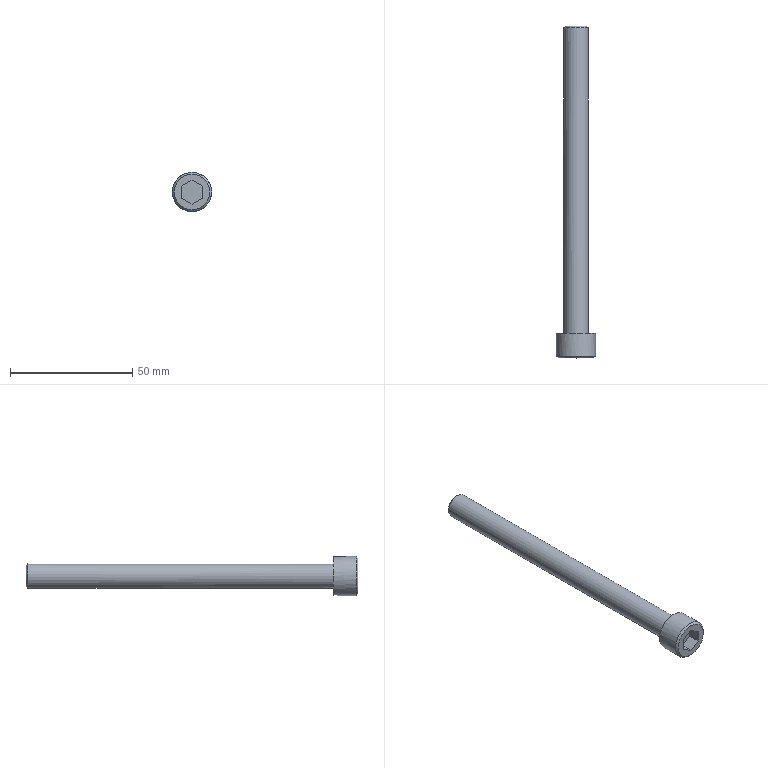Part | NX | features M10.00-135.00 2 | 1 solid | 14 faces | box 16 x 135.5 x 16 mm | volume 11532 mm3 | plane 10 | cylinder 2 | cone 2 | commonest cylinder face diameters 10 x1 16 x1
STEP:
#1=CARTESIAN_POINT('',(60.,-290.5,-15.25));
#2=VERTEX_POINT('',#1);
#3=CARTESIAN_POINT('',(60.,-290.5,-22.5));
#4=DIRECTION('',(0.,1.,0.));
#5=DIRECTION('',(0.,0.,1.));
#6=AXIS2_PLACEMENT_3D('',#3,#4,#5);
#7=CIRCLE('',#6,7.25);
#8=EDGE_CURVE('',#2,#2,#7,.T.);
#9=ORIENTED_EDGE('',*,*,#8,.F.);
#10=EDGE_LOOP('',(#9));
#11=FACE_BOUND('',#10,.T.);
#12=CARTESIAN_POINT('',(55.75,-290.5,-24.954));
#13=VERTEX_POINT('',#12);
#14=CARTESIAN_POINT('',(55.75,-290.5,-20.046));
#15=VERTEX_POINT('',#14);
#16=CARTESIAN_POINT('',(55.75,-290.5,-24.954));
#17=DIRECTION('',(0.,0.,1.));
#18=VECTOR('',#17,1000.);
#19=LINE('',#16,#18);
#20=EDGE_CURVE('',#13,#15,#19,.T.);
#21=ORIENTED_EDGE('',*,*,#20,.T.);
#22=CARTESIAN_POINT('',(60.,-290.5,-17.593));
#23=VERTEX_POINT('',#22);
#24=CARTESIAN_POINT('',(55.75,-290.5,-20.046));
#25=DIRECTION('',(0.866,0.,0.5));
#26=VECTOR('',#25,1000.);
#27=LINE('',#24,#26);
#28=EDGE_CURVE('',#15,#23,#27,.T.);
#29=ORIENTED_EDGE('',*,*,#28,.T.);
#30=CARTESIAN_POINT('',(64.25,-290.5,-20.046));
#31=VERTEX_POINT('',#30);
#32=CARTESIAN_POINT('',(60.,-290.5,-17.593));
#33=DIRECTION('',(0.866,0.,-0.5));
#34=VECTOR('',#33,1000.);
#35=LINE('',#32,#34);
#36=EDGE_CURVE('',#23,#31,#35,.T.);
#37=ORIENTED_EDGE('',*,*,#36,.T.);
#38=CARTESIAN_POINT('',(64.25,-290.5,-24.954));
#39=VERTEX_POINT('',#38);
#40=CARTESIAN_POINT('',(64.25,-290.5,-20.046));
#41=DIRECTION('',(0.,0.,-1.));
#42=VECTOR('',#41,1000.);
#43=LINE('',#40,#42);
#44=EDGE_CURVE('',#31,#39,#43,.T.);
#45=ORIENTED_EDGE('',*,*,#44,.T.);
#46=CARTESIAN_POINT('',(60.,-290.5,-27.407));
#47=VERTEX_POINT('',#46);
#48=CARTESIAN_POINT('',(64.25,-290.5,-24.954));
#49=DIRECTION('',(-0.866,0.,-0.5));
#50=VECTOR('',#49,1000.);
#51=LINE('',#48,#50);
#52=EDGE_CURVE('',#39,#47,#51,.T.);
#53=ORIENTED_EDGE('',*,*,#52,.T.);
#54=CARTESIAN_POINT('',(60.,-290.5,-27.407));
#55=DIRECTION('',(-0.866,0.,0.5));
#56=VECTOR('',#55,1000.);
#57=LINE('',#54,#56);
#58=EDGE_CURVE('',#47,#13,#57,.T.);
#59=ORIENTED_EDGE('',*,*,#58,.T.);
#60=EDGE_LOOP('',(#21,#29,#37,#45,#53,#59));
#61=FACE_BOUND('',#60,.T.);
#62=CARTESIAN_POINT('',(60.,-290.5,-22.5));
#63=DIRECTION('',(0.,-1.,0.));
#64=DIRECTION('',(0.,0.,1.));
#65=AXIS2_PLACEMENT_3D('',#62,#63,#64);
#66=PLANE('',#65);
#67=ADVANCED_FACE('',(#11,#61),#66,.T.);
#68=CARTESIAN_POINT('',(65.,-280.5,-22.5));
#69=VERTEX_POINT('',#68);
#70=CARTESIAN_POINT('',(60.,-280.5,-22.5));
#71=DIRECTION('',(0.,-1.,0.));
#72=DIRECTION('',(1.,0.,0.));
#73=AXIS2_PLACEMENT_3D('',#70,#71,#72);
#74=CIRCLE('',#73,5.);
#75=EDGE_CURVE('',#69,#69,#74,.T.);
#76=ORIENTED_EDGE('',*,*,#75,.T.);
#77=EDGE_LOOP('',(#76));
#78=FACE_BOUND('',#77,.T.);
#79=CARTESIAN_POINT('',(68.,-280.5,-22.5));
#80=VERTEX_POINT('',#79);
#81=CARTESIAN_POINT('',(60.,-280.5,-22.5));
#82=DIRECTION('',(0.,1.,0.));
#83=DIRECTION('',(1.,0.,0.));
#84=AXIS2_PLACEMENT_3D('',#81,#82,#83);
#85=CIRCLE('',#84,8.);
#86=EDGE_CURVE('',#80,#80,#85,.T.);
#87=ORIENTED_EDGE('',*,*,#86,.T.);
#88=EDGE_LOOP('',(#87));
#89=FACE_BOUND('',#88,.T.);
#90=CARTESIAN_POINT('',(60.,-280.5,-22.5));
#91=DIRECTION('',(0.,1.,0.));
#92=DIRECTION('',(0.,0.,-1.));
#93=AXIS2_PLACEMENT_3D('',#90,#91,#92);
#94=PLANE('',#93);
#95=ADVANCED_FACE('',(#78,#89),#94,.T.);
#96=CARTESIAN_POINT('',(60.,-289.75,-14.5));
#97=VERTEX_POINT('',#96);
#98=CARTESIAN_POINT('',(60.,-289.75,-22.5));
#99=DIRECTION('',(0.,1.,0.));
#100=DIRECTION('',(0.,0.,1.));
#101=AXIS2_PLACEMENT_3D('',#98,#99,#100);
#102=CIRCLE('',#101,8.);
#103=EDGE_CURVE('',#97,#97,#102,.F.);
#104=ORIENTED_EDGE('',*,*,#103,.F.);
#105=EDGE_LOOP('',(#104));
#106=FACE_BOUND('',#105,.T.);
#107=ORIENTED_EDGE('',*,*,#86,.F.);
#108=EDGE_LOOP('',(#107));
#109=FACE_BOUND('',#108,.T.);
#110=CARTESIAN_POINT('',(60.,-280.5,-22.5));
#111=DIRECTION('',(0.,-1.,0.));
#112=DIRECTION('',(1.,0.,0.));
#113=AXIS2_PLACEMENT_3D('',#110,#111,#112);
#114=CYLINDRICAL_SURFACE('',#113,8.);
#115=ADVANCED_FACE('',(#106,#109),#114,.T.);
#116=CARTESIAN_POINT('',(60.,-155.,-26.75));
#117=VERTEX_POINT('',#116);
#118=CARTESIAN_POINT('',(60.,-155.,-22.5));
#119=DIRECTION('',(0.,-1.,0.));
#120=DIRECTION('',(0.,0.,-1.));
#121=AXIS2_PLACEMENT_3D('',#118,#119,#120);
#122=CIRCLE('',#121,4.25);
#123=EDGE_CURVE('',#117,#117,#122,.T.);
#124=ORIENTED_EDGE('',*,*,#123,.F.);
#125=EDGE_LOOP('',(#124));
#126=FACE_BOUND('',#125,.T.);
#127=CARTESIAN_POINT('',(60.,-155.,-22.5));
#128=DIRECTION('',(0.,1.,0.));
#129=DIRECTION('',(0.,0.,-1.));
#130=AXIS2_PLACEMENT_3D('',#127,#128,#129);
#131=PLANE('',#130);
#132=ADVANCED_FACE('',(#126),#131,.T.);
#133=CARTESIAN_POINT('',(60.,-155.75,-27.5));
#134=VERTEX_POINT('',#133);
#135=CARTESIAN_POINT('',(60.,-155.75,-22.5));
#136=DIRECTION('',(0.,-1.,0.));
#137=DIRECTION('',(0.,0.,-1.));
#138=AXIS2_PLACEMENT_3D('',#135,#136,#137);
#139=CIRCLE('',#138,5.);
#140=EDGE_CURVE('',#134,#134,#139,.F.);
#141=ORIENTED_EDGE('',*,*,#140,.F.);
#142=EDGE_LOOP('',(#141));
#143=FACE_BOUND('',#142,.T.);
#144=ORIENTED_EDGE('',*,*,#75,.F.);
#145=EDGE_LOOP('',(#144));
#146=FACE_BOUND('',#145,.T.);
#147=CARTESIAN_POINT('',(60.,-280.5,-22.5));
#148=DIRECTION('',(0.,1.,0.));
#149=DIRECTION('',(1.,0.,0.));
#150=AXIS2_PLACEMENT_3D('',#147,#148,#149);
#151=CYLINDRICAL_SURFACE('',#150,5.);
#152=ADVANCED_FACE('',(#143,#146),#151,.T.);
#153=ORIENTED_EDGE('',*,*,#28,.F.);
#154=CARTESIAN_POINT('',(55.75,-285.5,-20.046));
#155=VERTEX_POINT('',#154);
#156=CARTESIAN_POINT('',(55.75,-285.5,-20.046));
#157=DIRECTION('',(0.,-1.,0.));
#158=VECTOR('',#157,1000.);
#159=LINE('',#156,#158);
#160=EDGE_CURVE('',#15,#155,#159,.F.);
#161=ORIENTED_EDGE('',*,*,#160,.T.);
#162=CARTESIAN_POINT('',(60.,-285.5,-17.593));
#163=VERTEX_POINT('',#162);
#164=CARTESIAN_POINT('',(55.75,-285.5,-20.046));
#165=DIRECTION('',(0.866,0.,0.5));
#166=VECTOR('',#165,1000.);
#167=LINE('',#164,#166);
#168=EDGE_CURVE('',#163,#155,#167,.F.);
#169=ORIENTED_EDGE('',*,*,#168,.F.);
#170=CARTESIAN_POINT('',(60.,-285.5,-17.593));
#171=DIRECTION('',(0.,-1.,0.));
#172=VECTOR('',#171,1000.);
#173=LINE('',#170,#172);
#174=EDGE_CURVE('',#23,#163,#173,.F.);
#175=ORIENTED_EDGE('',*,*,#174,.F.);
#176=EDGE_LOOP('',(#153,#161,#169,#175));
#177=FACE_BOUND('',#176,.T.);
#178=CARTESIAN_POINT('',(57.875,-288.,-18.819));
#179=DIRECTION('',(-0.5,0.,0.866));
#180=DIRECTION('',(0.866,0.,0.5));
#181=AXIS2_PLACEMENT_3D('',#178,#179,#180);
#182=PLANE('',#181);
#183=ADVANCED_FACE('',(#177),#182,.F.);
#184=ORIENTED_EDGE('',*,*,#20,.F.);
#185=CARTESIAN_POINT('',(55.75,-285.5,-24.954));
#186=VERTEX_POINT('',#185);
#187=CARTESIAN_POINT('',(55.75,-285.5,-24.954));
#188=DIRECTION('',(0.,-1.,0.));
#189=VECTOR('',#188,1000.);
#190=LINE('',#187,#189);
#191=EDGE_CURVE('',#13,#186,#190,.F.);
#192=ORIENTED_EDGE('',*,*,#191,.T.);
#193=CARTESIAN_POINT('',(55.75,-285.5,-24.954));
#194=DIRECTION('',(0.,0.,1.));
#195=VECTOR('',#194,1000.);
#196=LINE('',#193,#195);
#197=EDGE_CURVE('',#155,#186,#196,.F.);
#198=ORIENTED_EDGE('',*,*,#197,.F.);
#199=ORIENTED_EDGE('',*,*,#160,.F.);
#200=EDGE_LOOP('',(#184,#192,#198,#199));
#201=FACE_BOUND('',#200,.T.);
#202=CARTESIAN_POINT('',(55.75,-288.,-22.5));
#203=DIRECTION('',(-1.,0.,0.));
#204=DIRECTION('',(0.,1.,0.));
#205=AXIS2_PLACEMENT_3D('',#202,#203,#204);
#206=PLANE('',#205);
#207=ADVANCED_FACE('',(#201),#206,.F.);
#208=ORIENTED_EDGE('',*,*,#58,.F.);
#209=CARTESIAN_POINT('',(60.,-285.5,-27.407));
#210=VERTEX_POINT('',#209);
#211=CARTESIAN_POINT('',(60.,-285.5,-27.407));
#212=DIRECTION('',(0.,-1.,0.));
#213=VECTOR('',#212,1000.);
#214=LINE('',#211,#213);
#215=EDGE_CURVE('',#47,#210,#214,.F.);
#216=ORIENTED_EDGE('',*,*,#215,.T.);
#217=CARTESIAN_POINT('',(60.,-285.5,-27.407));
#218=DIRECTION('',(-0.866,0.,0.5));
#219=VECTOR('',#218,1000.);
#220=LINE('',#217,#219);
#221=EDGE_CURVE('',#186,#210,#220,.F.);
#222=ORIENTED_EDGE('',*,*,#221,.F.);
#223=ORIENTED_EDGE('',*,*,#191,.F.);
#224=EDGE_LOOP('',(#208,#216,#222,#223));
#225=FACE_BOUND('',#224,.T.);
#226=CARTESIAN_POINT('',(57.875,-288.,-26.181));
#227=DIRECTION('',(-0.5,0.,-0.866));
#228=DIRECTION('',(-0.866,0.,0.5));
#229=AXIS2_PLACEMENT_3D('',#226,#227,#228);
#230=PLANE('',#229);
#231=ADVANCED_FACE('',(#225),#230,.F.);
#232=ORIENTED_EDGE('',*,*,#52,.F.);
#233=CARTESIAN_POINT('',(64.25,-285.5,-24.954));
#234=VERTEX_POINT('',#233);
#235=CARTESIAN_POINT('',(64.25,-285.5,-24.954));
#236=DIRECTION('',(0.,-1.,0.));
#237=VECTOR('',#236,1000.);
#238=LINE('',#235,#237);
#239=EDGE_CURVE('',#39,#234,#238,.F.);
#240=ORIENTED_EDGE('',*,*,#239,.T.);
#241=CARTESIAN_POINT('',(64.25,-285.5,-24.954));
#242=DIRECTION('',(-0.866,0.,-0.5));
#243=VECTOR('',#242,1000.);
#244=LINE('',#241,#243);
#245=EDGE_CURVE('',#210,#234,#244,.F.);
#246=ORIENTED_EDGE('',*,*,#245,.F.);
#247=ORIENTED_EDGE('',*,*,#215,.F.);
#248=EDGE_LOOP('',(#232,#240,#246,#247));
#249=FACE_BOUND('',#248,.T.);
#250=CARTESIAN_POINT('',(62.125,-288.,-26.181));
#251=DIRECTION('',(0.5,0.,-0.866));
#252=DIRECTION('',(-0.866,0.,-0.5));
#253=AXIS2_PLACEMENT_3D('',#250,#251,#252);
#254=PLANE('',#253);
#255=ADVANCED_FACE('',(#249),#254,.F.);
#256=ORIENTED_EDGE('',*,*,#44,.F.);
#257=CARTESIAN_POINT('',(64.25,-285.5,-20.046));
#258=VERTEX_POINT('',#257);
#259=CARTESIAN_POINT('',(64.25,-285.5,-20.046));
#260=DIRECTION('',(0.,-1.,0.));
#261=VECTOR('',#260,1000.);
#262=LINE('',#259,#261);
#263=EDGE_CURVE('',#31,#258,#262,.F.);
#264=ORIENTED_EDGE('',*,*,#263,.T.);
#265=CARTESIAN_POINT('',(64.25,-285.5,-20.046));
#266=DIRECTION('',(0.,0.,-1.));
#267=VECTOR('',#266,1000.);
#268=LINE('',#265,#267);
#269=EDGE_CURVE('',#234,#258,#268,.F.);
#270=ORIENTED_EDGE('',*,*,#269,.F.);
#271=ORIENTED_EDGE('',*,*,#239,.F.);
#272=EDGE_LOOP('',(#256,#264,#270,#271));
#273=FACE_BOUND('',#272,.T.);
#274=CARTESIAN_POINT('',(64.25,-288.,-22.5));
#275=DIRECTION('',(1.,0.,0.));
#276=DIRECTION('',(0.,-1.,0.));
#277=AXIS2_PLACEMENT_3D('',#274,#275,#276);
#278=PLANE('',#277);
#279=ADVANCED_FACE('',(#273),#278,.F.);
#280=ORIENTED_EDGE('',*,*,#36,.F.);
#281=ORIENTED_EDGE('',*,*,#174,.T.);
#282=CARTESIAN_POINT('',(60.,-285.5,-17.593));
#283=DIRECTION('',(0.866,0.,-0.5));
#284=VECTOR('',#283,1000.);
#285=LINE('',#282,#284);
#286=EDGE_CURVE('',#258,#163,#285,.F.);
#287=ORIENTED_EDGE('',*,*,#286,.F.);
#288=ORIENTED_EDGE('',*,*,#263,.F.);
#289=EDGE_LOOP('',(#280,#281,#287,#288));
#290=FACE_BOUND('',#289,.T.);
#291=CARTESIAN_POINT('',(62.125,-288.,-18.819));
#292=DIRECTION('',(0.5,0.,0.866));
#293=DIRECTION('',(0.866,0.,-0.5));
#294=AXIS2_PLACEMENT_3D('',#291,#292,#293);
#295=PLANE('',#294);
#296=ADVANCED_FACE('',(#290),#295,.F.);
#297=ORIENTED_EDGE('',*,*,#286,.T.);
#298=ORIENTED_EDGE('',*,*,#168,.T.);
#299=ORIENTED_EDGE('',*,*,#197,.T.);
#300=ORIENTED_EDGE('',*,*,#221,.T.);
#301=ORIENTED_EDGE('',*,*,#245,.T.);
#302=ORIENTED_EDGE('',*,*,#269,.T.);
#303=EDGE_LOOP('',(#297,#298,#299,#300,#301,#302));
#304=FACE_BOUND('',#303,.T.);
#305=CARTESIAN_POINT('',(60.,-285.5,-22.5));
#306=DIRECTION('',(0.,1.,0.));
#307=DIRECTION('',(0.,0.,-1.));
#308=AXIS2_PLACEMENT_3D('',#305,#306,#307);
#309=PLANE('',#308);
#310=ADVANCED_FACE('',(#304),#309,.F.);
#311=ORIENTED_EDGE('',*,*,#123,.T.);
#312=EDGE_LOOP('',(#311));
#313=FACE_BOUND('',#312,.T.);
#314=ORIENTED_EDGE('',*,*,#140,.T.);
#315=EDGE_LOOP('',(#314));
#316=FACE_BOUND('',#315,.T.);
#317=CARTESIAN_POINT('',(60.,-155.75,-22.5));
#318=DIRECTION('',(0.,-1.,0.));
#319=DIRECTION('',(0.,0.,1.));
#320=AXIS2_PLACEMENT_3D('',#317,#318,#319);
#321=CONICAL_SURFACE('',#320,5.,0.7854);
#322=ADVANCED_FACE('',(#313,#316),#321,.T.);
#323=ORIENTED_EDGE('',*,*,#8,.T.);
#324=EDGE_LOOP('',(#323));
#325=FACE_BOUND('',#324,.T.);
#326=ORIENTED_EDGE('',*,*,#103,.T.);
#327=EDGE_LOOP('',(#326));
#328=FACE_BOUND('',#327,.T.);
#329=CARTESIAN_POINT('',(60.,-289.75,-22.5));
#330=DIRECTION('',(0.,1.,0.));
#331=DIRECTION('',(0.,0.,-1.));
#332=AXIS2_PLACEMENT_3D('',#329,#330,#331);
#333=CONICAL_SURFACE('',#332,8.,0.7854);
#334=ADVANCED_FACE('',(#325,#328),#333,.T.);
#335=CLOSED_SHELL('',(#67,#95,#115,#132,#152,#183,#207,#231,#255,#279,#296,#310,#322,#334));
#336=MANIFOLD_SOLID_BREP('',#335);
#337=(LENGTH_UNIT()NAMED_UNIT(*)SI_UNIT(.MILLI.,.METRE.));
#338=UNCERTAINTY_MEASURE_WITH_UNIT(LENGTH_MEASURE(0.00001),#337,'','');
#339=(NAMED_UNIT(*)PLANE_ANGLE_UNIT()SI_UNIT($,.RADIAN.));
#340=(NAMED_UNIT(*)SI_UNIT($,.STERADIAN.)SOLID_ANGLE_UNIT());
#341=(GEOMETRIC_REPRESENTATION_CONTEXT(3)GLOBAL_UNCERTAINTY_ASSIGNED_CONTEXT((#338))GLOBAL_UNIT_ASSIGNED_CONTEXT((#337,#339,#340))REPRESENTATION_CONTEXT('',''));
#342=ADVANCED_BREP_SHAPE_REPRESENTATION('',(#336),#341);